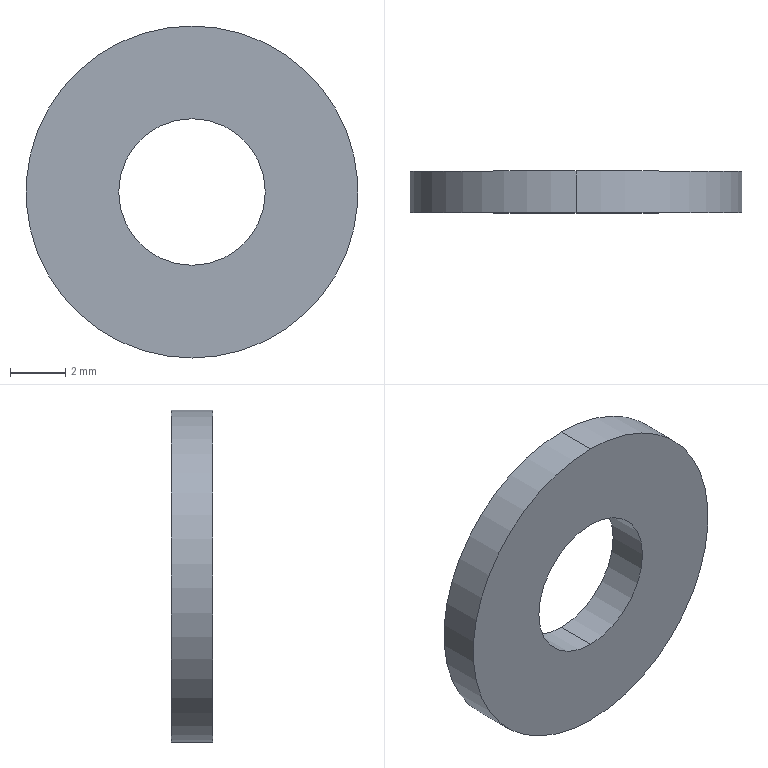Part | SolidWorks | features FlatPattern 1, SMBaseFlange 1, SheetMetal 1 | 1 solid | 6 faces | box 12 x 1.5 x 12 mm | volume 136.553 mm3 | cylinder 4 | plane 2 | commonest cylinder face diameters 5.3 x2 12 x2
STEP:
#1=CARTESIAN_POINT('',(0.,-1.5,-2.65));
#2=VERTEX_POINT('',#1);
#3=CARTESIAN_POINT('',(0.,-1.5,2.65));
#4=VERTEX_POINT('',#3);
#5=CARTESIAN_POINT('',(0.,-1.5,0.));
#6=DIRECTION('',(0.,1.,0.));
#7=DIRECTION('',(0.,0.,1.));
#8=AXIS2_PLACEMENT_3D('',#5,#6,#7);
#9=CIRCLE('',#8,2.65);
#10=EDGE_CURVE('',#2,#4,#9,.T.);
#11=ORIENTED_EDGE('',*,*,#10,.F.);
#12=CARTESIAN_POINT('',(0.,0.,-2.65));
#13=VERTEX_POINT('',#12);
#14=CARTESIAN_POINT('',(0.,-1.5,-2.65));
#15=DIRECTION('',(0.,1.,0.));
#16=VECTOR('',#15,1000.);
#17=LINE('',#14,#16);
#18=EDGE_CURVE('',#2,#13,#17,.T.);
#19=ORIENTED_EDGE('',*,*,#18,.T.);
#20=CARTESIAN_POINT('',(0.,0.,2.65));
#21=VERTEX_POINT('',#20);
#22=CARTESIAN_POINT('',(0.,0.,0.));
#23=DIRECTION('',(0.,1.,0.));
#24=DIRECTION('',(0.,0.,1.));
#25=AXIS2_PLACEMENT_3D('',#22,#23,#24);
#26=CIRCLE('',#25,2.65);
#27=EDGE_CURVE('',#13,#21,#26,.T.);
#28=ORIENTED_EDGE('',*,*,#27,.T.);
#29=CARTESIAN_POINT('',(0.,-1.5,2.65));
#30=DIRECTION('',(0.,1.,0.));
#31=VECTOR('',#30,1000.);
#32=LINE('',#29,#31);
#33=EDGE_CURVE('',#4,#21,#32,.T.);
#34=ORIENTED_EDGE('',*,*,#33,.F.);
#35=EDGE_LOOP('',(#11,#19,#28,#34));
#36=FACE_OUTER_BOUND('',#35,.T.);
#37=CARTESIAN_POINT('',(0.,-1.5,0.));
#38=DIRECTION('',(0.,1.,0.));
#39=DIRECTION('',(0.,0.,1.));
#40=AXIS2_PLACEMENT_3D('',#37,#38,#39);
#41=CYLINDRICAL_SURFACE('',#40,2.65);
#42=ADVANCED_FACE('',(#36),#41,.F.);
#43=CARTESIAN_POINT('',(0.,-1.5,6.));
#44=VERTEX_POINT('',#43);
#45=CARTESIAN_POINT('',(0.,-1.5,-6.));
#46=VERTEX_POINT('',#45);
#47=CARTESIAN_POINT('',(0.,-1.5,0.));
#48=DIRECTION('',(0.,1.,0.));
#49=DIRECTION('',(0.,0.,1.));
#50=AXIS2_PLACEMENT_3D('',#47,#48,#49);
#51=CIRCLE('',#50,6.);
#52=EDGE_CURVE('',#44,#46,#51,.T.);
#53=ORIENTED_EDGE('',*,*,#52,.T.);
#54=CARTESIAN_POINT('',(0.,0.,-6.));
#55=VERTEX_POINT('',#54);
#56=CARTESIAN_POINT('',(0.,-1.5,-6.));
#57=DIRECTION('',(0.,1.,0.));
#58=VECTOR('',#57,1000.);
#59=LINE('',#56,#58);
#60=EDGE_CURVE('',#46,#55,#59,.T.);
#61=ORIENTED_EDGE('',*,*,#60,.T.);
#62=CARTESIAN_POINT('',(0.,0.,6.));
#63=VERTEX_POINT('',#62);
#64=CARTESIAN_POINT('',(0.,0.,0.));
#65=DIRECTION('',(0.,1.,0.));
#66=DIRECTION('',(0.,0.,1.));
#67=AXIS2_PLACEMENT_3D('',#64,#65,#66);
#68=CIRCLE('',#67,6.);
#69=EDGE_CURVE('',#63,#55,#68,.T.);
#70=ORIENTED_EDGE('',*,*,#69,.F.);
#71=CARTESIAN_POINT('',(0.,-1.5,6.));
#72=DIRECTION('',(0.,1.,0.));
#73=VECTOR('',#72,1000.);
#74=LINE('',#71,#73);
#75=EDGE_CURVE('',#44,#63,#74,.T.);
#76=ORIENTED_EDGE('',*,*,#75,.F.);
#77=EDGE_LOOP('',(#53,#61,#70,#76));
#78=FACE_OUTER_BOUND('',#77,.T.);
#79=CARTESIAN_POINT('',(0.,-1.5,0.));
#80=DIRECTION('',(0.,1.,0.));
#81=DIRECTION('',(0.,0.,1.));
#82=AXIS2_PLACEMENT_3D('',#79,#80,#81);
#83=CYLINDRICAL_SURFACE('',#82,6.);
#84=ADVANCED_FACE('',(#78),#83,.T.);
#85=ORIENTED_EDGE('',*,*,#60,.F.);
#86=CARTESIAN_POINT('',(0.,-1.5,0.));
#87=DIRECTION('',(0.,1.,0.));
#88=DIRECTION('',(0.,0.,1.));
#89=AXIS2_PLACEMENT_3D('',#86,#87,#88);
#90=CIRCLE('',#89,6.);
#91=EDGE_CURVE('',#46,#44,#90,.T.);
#92=ORIENTED_EDGE('',*,*,#91,.T.);
#93=ORIENTED_EDGE('',*,*,#75,.T.);
#94=CARTESIAN_POINT('',(0.,0.,0.));
#95=DIRECTION('',(0.,1.,0.));
#96=DIRECTION('',(0.,0.,1.));
#97=AXIS2_PLACEMENT_3D('',#94,#95,#96);
#98=CIRCLE('',#97,6.);
#99=EDGE_CURVE('',#55,#63,#98,.T.);
#100=ORIENTED_EDGE('',*,*,#99,.F.);
#101=EDGE_LOOP('',(#85,#92,#93,#100));
#102=FACE_OUTER_BOUND('',#101,.T.);
#103=CARTESIAN_POINT('',(0.,-1.5,0.));
#104=DIRECTION('',(0.,1.,0.));
#105=DIRECTION('',(0.,0.,1.));
#106=AXIS2_PLACEMENT_3D('',#103,#104,#105);
#107=CYLINDRICAL_SURFACE('',#106,6.);
#108=ADVANCED_FACE('',(#102),#107,.T.);
#109=CARTESIAN_POINT('',(0.,-1.5,0.));
#110=DIRECTION('',(0.,1.,0.));
#111=DIRECTION('',(0.,0.,1.));
#112=AXIS2_PLACEMENT_3D('',#109,#110,#111);
#113=CIRCLE('',#112,2.65);
#114=EDGE_CURVE('',#4,#2,#113,.T.);
#115=ORIENTED_EDGE('',*,*,#114,.T.);
#116=ORIENTED_EDGE('',*,*,#10,.T.);
#117=EDGE_LOOP('',(#115,#116));
#118=FACE_BOUND('',#117,.T.);
#119=ORIENTED_EDGE('',*,*,#52,.F.);
#120=ORIENTED_EDGE('',*,*,#91,.F.);
#121=EDGE_LOOP('',(#119,#120));
#122=FACE_OUTER_BOUND('',#121,.T.);
#123=CARTESIAN_POINT('',(0.,-1.5,0.));
#124=DIRECTION('',(0.,1.,0.));
#125=DIRECTION('',(0.,0.,1.));
#126=AXIS2_PLACEMENT_3D('',#123,#124,#125);
#127=PLANE('',#126);
#128=ADVANCED_FACE('',(#118,#122),#127,.F.);
#129=CARTESIAN_POINT('',(0.,0.,0.));
#130=DIRECTION('',(0.,1.,0.));
#131=DIRECTION('',(0.,0.,1.));
#132=AXIS2_PLACEMENT_3D('',#129,#130,#131);
#133=CIRCLE('',#132,2.65);
#134=EDGE_CURVE('',#21,#13,#133,.T.);
#135=ORIENTED_EDGE('',*,*,#134,.F.);
#136=ORIENTED_EDGE('',*,*,#27,.F.);
#137=EDGE_LOOP('',(#135,#136));
#138=FACE_BOUND('',#137,.T.);
#139=ORIENTED_EDGE('',*,*,#69,.T.);
#140=ORIENTED_EDGE('',*,*,#99,.T.);
#141=EDGE_LOOP('',(#139,#140));
#142=FACE_OUTER_BOUND('',#141,.T.);
#143=CARTESIAN_POINT('',(0.,0.,0.));
#144=DIRECTION('',(0.,1.,0.));
#145=DIRECTION('',(0.,0.,1.));
#146=AXIS2_PLACEMENT_3D('',#143,#144,#145);
#147=PLANE('',#146);
#148=ADVANCED_FACE('',(#138,#142),#147,.T.);
#149=ORIENTED_EDGE('',*,*,#18,.F.);
#150=ORIENTED_EDGE('',*,*,#114,.F.);
#151=ORIENTED_EDGE('',*,*,#33,.T.);
#152=ORIENTED_EDGE('',*,*,#134,.T.);
#153=EDGE_LOOP('',(#149,#150,#151,#152));
#154=FACE_OUTER_BOUND('',#153,.T.);
#155=CARTESIAN_POINT('',(0.,-1.5,0.));
#156=DIRECTION('',(0.,1.,0.));
#157=DIRECTION('',(0.,0.,1.));
#158=AXIS2_PLACEMENT_3D('',#155,#156,#157);
#159=CYLINDRICAL_SURFACE('',#158,2.65);
#160=ADVANCED_FACE('',(#154),#159,.F.);
#161=CLOSED_SHELL('',(#42,#84,#108,#128,#148,#160));
#162=MANIFOLD_SOLID_BREP('',#161);
#163=CARTESIAN_POINT('',(0.,0.,0.));
#164=DIRECTION('',(0.,0.,1.));
#165=DIRECTION('',(1.,0.,0.));
#166=AXIS2_PLACEMENT_3D('',#163,#164,#165);
#167=(LENGTH_UNIT()NAMED_UNIT(*)SI_UNIT(.MILLI.,.METRE.));
#168=UNCERTAINTY_MEASURE_WITH_UNIT(LENGTH_MEASURE(0.00001),#167,'','');
#169=(NAMED_UNIT(*)PLANE_ANGLE_UNIT()SI_UNIT($,.RADIAN.));
#170=(NAMED_UNIT(*)SI_UNIT($,.STERADIAN.)SOLID_ANGLE_UNIT());
#171=(GEOMETRIC_REPRESENTATION_CONTEXT(3)GLOBAL_UNCERTAINTY_ASSIGNED_CONTEXT((#168))GLOBAL_UNIT_ASSIGNED_CONTEXT((#167,#169,#170))REPRESENTATION_CONTEXT('',''));
#172=ADVANCED_BREP_SHAPE_REPRESENTATION('',(#162,#166),#171);